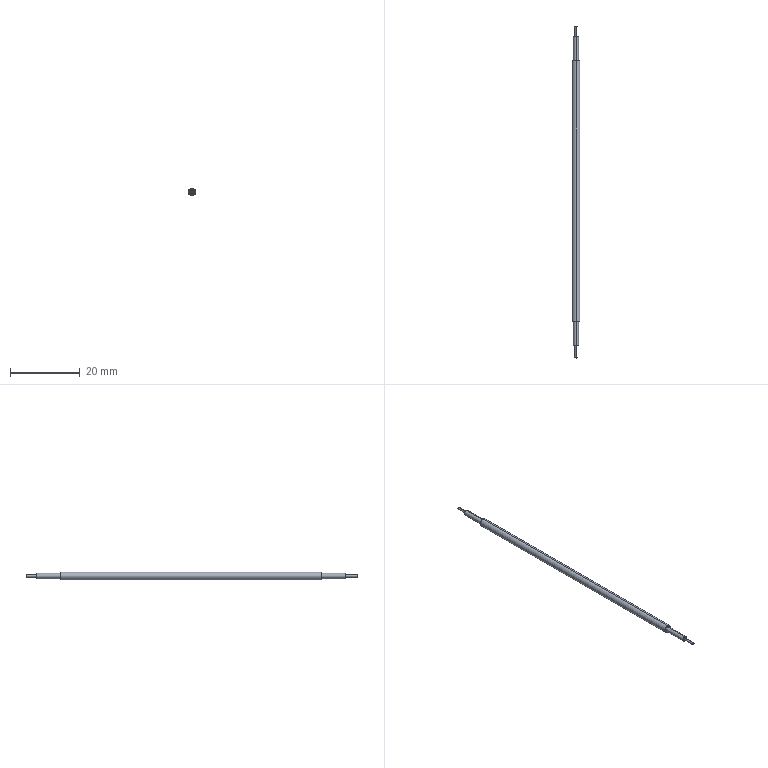Part | SolidWorks | features ICE 4, Extrusion 1 | 1 solid | 16 faces | box 2.25 x 95.2 x 2.25 mm | volume 323.59 mm3 | cylinder 10 | plane 6 | commonest cylinder face diameters 0.6 x4 1.5 x4 2.25 x2
STEP:
#1=CARTESIAN_POINT('',(0.,84.7,0.2999));
#2=VERTEX_POINT('',#1);
#3=CARTESIAN_POINT('',(0.,84.7,-0.2999));
#4=VERTEX_POINT('',#3);
#5=CARTESIAN_POINT('',(0.,84.7,0.));
#6=DIRECTION('',(0.,1.,0.));
#7=DIRECTION('',(0.,0.,1.));
#8=AXIS2_PLACEMENT_3D('',#5,#6,#7);
#9=CIRCLE('',#8,0.2999);
#10=EDGE_CURVE('',#2,#4,#9,.T.);
#11=ORIENTED_EDGE('',*,*,#10,.F.);
#12=CARTESIAN_POINT('',(0.,81.7,0.2999));
#13=VERTEX_POINT('',#12);
#14=CARTESIAN_POINT('',(0.,84.7,0.2999));
#15=DIRECTION('',(0.,-1.,0.));
#16=VECTOR('',#15,1000.);
#17=LINE('',#14,#16);
#18=EDGE_CURVE('',#2,#13,#17,.T.);
#19=ORIENTED_EDGE('',*,*,#18,.T.);
#20=CARTESIAN_POINT('',(0.,81.7,-0.2999));
#21=VERTEX_POINT('',#20);
#22=CARTESIAN_POINT('',(0.,81.7,0.));
#23=DIRECTION('',(0.,1.,0.));
#24=DIRECTION('',(0.,0.,1.));
#25=AXIS2_PLACEMENT_3D('',#22,#23,#24);
#26=CIRCLE('',#25,0.2999);
#27=EDGE_CURVE('',#13,#21,#26,.T.);
#28=ORIENTED_EDGE('',*,*,#27,.T.);
#29=CARTESIAN_POINT('',(0.,84.7,-0.2999));
#30=DIRECTION('',(0.,-1.,0.));
#31=VECTOR('',#30,1000.);
#32=LINE('',#29,#31);
#33=EDGE_CURVE('',#4,#21,#32,.T.);
#34=ORIENTED_EDGE('',*,*,#33,.F.);
#35=EDGE_LOOP('',(#11,#19,#28,#34));
#36=FACE_OUTER_BOUND('',#35,.T.);
#37=CARTESIAN_POINT('',(0.,84.7,0.));
#38=DIRECTION('',(0.,-1.,0.));
#39=DIRECTION('',(0.,0.,-1.));
#40=AXIS2_PLACEMENT_3D('',#37,#38,#39);
#41=CYLINDRICAL_SURFACE('',#40,0.2999);
#42=ADVANCED_FACE('',(#36),#41,.T.);
#43=CARTESIAN_POINT('',(0.,81.7,0.75));
#44=VERTEX_POINT('',#43);
#45=CARTESIAN_POINT('',(0.,81.7,-0.75));
#46=VERTEX_POINT('',#45);
#47=CARTESIAN_POINT('',(0.,81.7,0.));
#48=DIRECTION('',(0.,1.,0.));
#49=DIRECTION('',(0.,0.,1.));
#50=AXIS2_PLACEMENT_3D('',#47,#48,#49);
#51=CIRCLE('',#50,0.75);
#52=EDGE_CURVE('',#44,#46,#51,.T.);
#53=ORIENTED_EDGE('',*,*,#52,.F.);
#54=CARTESIAN_POINT('',(0.,74.7,0.75));
#55=VERTEX_POINT('',#54);
#56=CARTESIAN_POINT('',(0.,81.7,0.75));
#57=DIRECTION('',(0.,-1.,0.));
#58=VECTOR('',#57,1000.);
#59=LINE('',#56,#58);
#60=EDGE_CURVE('',#44,#55,#59,.T.);
#61=ORIENTED_EDGE('',*,*,#60,.T.);
#62=CARTESIAN_POINT('',(0.,74.7,-0.75));
#63=VERTEX_POINT('',#62);
#64=CARTESIAN_POINT('',(0.,74.7,0.));
#65=DIRECTION('',(0.,1.,0.));
#66=DIRECTION('',(0.,0.,1.));
#67=AXIS2_PLACEMENT_3D('',#64,#65,#66);
#68=CIRCLE('',#67,0.75);
#69=EDGE_CURVE('',#55,#63,#68,.T.);
#70=ORIENTED_EDGE('',*,*,#69,.T.);
#71=CARTESIAN_POINT('',(0.,81.7,-0.75));
#72=DIRECTION('',(0.,-1.,0.));
#73=VECTOR('',#72,1000.);
#74=LINE('',#71,#73);
#75=EDGE_CURVE('',#46,#63,#74,.T.);
#76=ORIENTED_EDGE('',*,*,#75,.F.);
#77=EDGE_LOOP('',(#53,#61,#70,#76));
#78=FACE_OUTER_BOUND('',#77,.T.);
#79=CARTESIAN_POINT('',(0.,81.7,0.));
#80=DIRECTION('',(0.,-1.,0.));
#81=DIRECTION('',(0.,0.,-1.));
#82=AXIS2_PLACEMENT_3D('',#79,#80,#81);
#83=CYLINDRICAL_SURFACE('',#82,0.75);
#84=ADVANCED_FACE('',(#78),#83,.T.);
#85=CARTESIAN_POINT('',(0.,-10.5,-0.3));
#86=VERTEX_POINT('',#85);
#87=CARTESIAN_POINT('',(0.,-10.5,0.3));
#88=VERTEX_POINT('',#87);
#89=CARTESIAN_POINT('',(0.,-10.5,0.));
#90=DIRECTION('',(0.,-1.,0.));
#91=DIRECTION('',(0.,0.,-1.));
#92=AXIS2_PLACEMENT_3D('',#89,#90,#91);
#93=CIRCLE('',#92,0.3);
#94=EDGE_CURVE('',#86,#88,#93,.T.);
#95=ORIENTED_EDGE('',*,*,#94,.F.);
#96=CARTESIAN_POINT('',(0.,-7.,-0.3));
#97=VERTEX_POINT('',#96);
#98=CARTESIAN_POINT('',(0.,-10.5,-0.3));
#99=DIRECTION('',(0.,1.,0.));
#100=VECTOR('',#99,1000.);
#101=LINE('',#98,#100);
#102=EDGE_CURVE('',#86,#97,#101,.T.);
#103=ORIENTED_EDGE('',*,*,#102,.T.);
#104=CARTESIAN_POINT('',(0.,-7.,0.3));
#105=VERTEX_POINT('',#104);
#106=CARTESIAN_POINT('',(0.,-7.,0.));
#107=DIRECTION('',(0.,-1.,0.));
#108=DIRECTION('',(0.,0.,-1.));
#109=AXIS2_PLACEMENT_3D('',#106,#107,#108);
#110=CIRCLE('',#109,0.3);
#111=EDGE_CURVE('',#97,#105,#110,.T.);
#112=ORIENTED_EDGE('',*,*,#111,.T.);
#113=CARTESIAN_POINT('',(0.,-10.5,0.3));
#114=DIRECTION('',(0.,1.,0.));
#115=VECTOR('',#114,1000.);
#116=LINE('',#113,#115);
#117=EDGE_CURVE('',#88,#105,#116,.T.);
#118=ORIENTED_EDGE('',*,*,#117,.F.);
#119=EDGE_LOOP('',(#95,#103,#112,#118));
#120=FACE_OUTER_BOUND('',#119,.T.);
#121=CARTESIAN_POINT('',(0.,-10.5,0.));
#122=DIRECTION('',(0.,1.,0.));
#123=DIRECTION('',(0.,0.,1.));
#124=AXIS2_PLACEMENT_3D('',#121,#122,#123);
#125=CYLINDRICAL_SURFACE('',#124,0.3);
#126=ADVANCED_FACE('',(#120),#125,.T.);
#127=CARTESIAN_POINT('',(0.,-7.,-0.75));
#128=VERTEX_POINT('',#127);
#129=CARTESIAN_POINT('',(0.,-7.,0.75));
#130=VERTEX_POINT('',#129);
#131=CARTESIAN_POINT('',(0.,-7.,0.));
#132=DIRECTION('',(0.,-1.,0.));
#133=DIRECTION('',(0.,0.,-1.));
#134=AXIS2_PLACEMENT_3D('',#131,#132,#133);
#135=CIRCLE('',#134,0.75);
#136=EDGE_CURVE('',#128,#130,#135,.T.);
#137=ORIENTED_EDGE('',*,*,#136,.F.);
#138=CARTESIAN_POINT('',(0.,0.,-0.75));
#139=VERTEX_POINT('',#138);
#140=CARTESIAN_POINT('',(0.,-7.,-0.75));
#141=DIRECTION('',(0.,1.,0.));
#142=VECTOR('',#141,1000.);
#143=LINE('',#140,#142);
#144=EDGE_CURVE('',#128,#139,#143,.T.);
#145=ORIENTED_EDGE('',*,*,#144,.T.);
#146=CARTESIAN_POINT('',(0.,0.,0.75));
#147=VERTEX_POINT('',#146);
#148=CARTESIAN_POINT('',(0.,0.,0.));
#149=DIRECTION('',(0.,-1.,0.));
#150=DIRECTION('',(0.,0.,1.));
#151=AXIS2_PLACEMENT_3D('',#148,#149,#150);
#152=CIRCLE('',#151,0.75);
#153=EDGE_CURVE('',#139,#147,#152,.T.);
#154=ORIENTED_EDGE('',*,*,#153,.T.);
#155=CARTESIAN_POINT('',(0.,-7.,0.75));
#156=DIRECTION('',(0.,1.,0.));
#157=VECTOR('',#156,1000.);
#158=LINE('',#155,#157);
#159=EDGE_CURVE('',#130,#147,#158,.T.);
#160=ORIENTED_EDGE('',*,*,#159,.F.);
#161=EDGE_LOOP('',(#137,#145,#154,#160));
#162=FACE_OUTER_BOUND('',#161,.T.);
#163=CARTESIAN_POINT('',(0.,-7.,0.));
#164=DIRECTION('',(0.,1.,0.));
#165=DIRECTION('',(0.,0.,1.));
#166=AXIS2_PLACEMENT_3D('',#163,#164,#165);
#167=CYLINDRICAL_SURFACE('',#166,0.75);
#168=ADVANCED_FACE('',(#162),#167,.T.);
#169=CARTESIAN_POINT('',(0.,74.7,1.125));
#170=VERTEX_POINT('',#169);
#171=CARTESIAN_POINT('',(0.,74.7,-1.125));
#172=VERTEX_POINT('',#171);
#173=CARTESIAN_POINT('',(0.,74.7,0.));
#174=DIRECTION('',(0.,1.,0.));
#175=DIRECTION('',(0.,0.,1.));
#176=AXIS2_PLACEMENT_3D('',#173,#174,#175);
#177=CIRCLE('',#176,1.125);
#178=EDGE_CURVE('',#170,#172,#177,.T.);
#179=ORIENTED_EDGE('',*,*,#178,.F.);
#180=CARTESIAN_POINT('',(0.,0.,1.125));
#181=VERTEX_POINT('',#180);
#182=CARTESIAN_POINT('',(0.,74.7,1.125));
#183=DIRECTION('',(0.,-1.,0.));
#184=VECTOR('',#183,1000.);
#185=LINE('',#182,#184);
#186=EDGE_CURVE('',#170,#181,#185,.T.);
#187=ORIENTED_EDGE('',*,*,#186,.T.);
#188=CARTESIAN_POINT('',(0.,0.,-1.125));
#189=VERTEX_POINT('',#188);
#190=CARTESIAN_POINT('',(0.,0.,0.));
#191=DIRECTION('',(0.,1.,0.));
#192=DIRECTION('',(0.,0.,1.));
#193=AXIS2_PLACEMENT_3D('',#190,#191,#192);
#194=CIRCLE('',#193,1.125);
#195=EDGE_CURVE('',#181,#189,#194,.T.);
#196=ORIENTED_EDGE('',*,*,#195,.T.);
#197=CARTESIAN_POINT('',(0.,74.7,-1.125));
#198=DIRECTION('',(0.,-1.,0.));
#199=VECTOR('',#198,1000.);
#200=LINE('',#197,#199);
#201=EDGE_CURVE('',#172,#189,#200,.T.);
#202=ORIENTED_EDGE('',*,*,#201,.F.);
#203=EDGE_LOOP('',(#179,#187,#196,#202));
#204=FACE_OUTER_BOUND('',#203,.T.);
#205=CARTESIAN_POINT('',(0.,74.7,0.));
#206=DIRECTION('',(0.,-1.,0.));
#207=DIRECTION('',(0.,0.,-1.));
#208=AXIS2_PLACEMENT_3D('',#205,#206,#207);
#209=CYLINDRICAL_SURFACE('',#208,1.125);
#210=ADVANCED_FACE('',(#204),#209,.T.);
#211=CARTESIAN_POINT('',(0.,81.7,0.));
#212=DIRECTION('',(0.,1.,0.));
#213=DIRECTION('',(0.,0.,1.));
#214=AXIS2_PLACEMENT_3D('',#211,#212,#213);
#215=CIRCLE('',#214,0.75);
#216=EDGE_CURVE('',#46,#44,#215,.T.);
#217=ORIENTED_EDGE('',*,*,#216,.T.);
#218=ORIENTED_EDGE('',*,*,#52,.T.);
#219=EDGE_LOOP('',(#217,#218));
#220=FACE_OUTER_BOUND('',#219,.T.);
#221=CARTESIAN_POINT('',(0.,81.7,0.));
#222=DIRECTION('',(0.,1.,0.));
#223=DIRECTION('',(0.,0.,1.));
#224=AXIS2_PLACEMENT_3D('',#221,#222,#223);
#225=CIRCLE('',#224,0.2999);
#226=EDGE_CURVE('',#21,#13,#225,.T.);
#227=ORIENTED_EDGE('',*,*,#226,.F.);
#228=ORIENTED_EDGE('',*,*,#27,.F.);
#229=EDGE_LOOP('',(#227,#228));
#230=FACE_BOUND('',#229,.T.);
#231=CARTESIAN_POINT('',(0.,81.7,0.));
#232=DIRECTION('',(0.,1.,0.));
#233=DIRECTION('',(0.,0.,1.));
#234=AXIS2_PLACEMENT_3D('',#231,#232,#233);
#235=PLANE('',#234);
#236=ADVANCED_FACE('',(#220,#230),#235,.T.);
#237=CARTESIAN_POINT('',(0.,74.7,0.));
#238=DIRECTION('',(0.,1.,0.));
#239=DIRECTION('',(0.,0.,1.));
#240=AXIS2_PLACEMENT_3D('',#237,#238,#239);
#241=CIRCLE('',#240,1.125);
#242=EDGE_CURVE('',#172,#170,#241,.T.);
#243=ORIENTED_EDGE('',*,*,#242,.T.);
#244=ORIENTED_EDGE('',*,*,#178,.T.);
#245=EDGE_LOOP('',(#243,#244));
#246=FACE_OUTER_BOUND('',#245,.T.);
#247=CARTESIAN_POINT('',(0.,74.7,0.));
#248=DIRECTION('',(0.,1.,0.));
#249=DIRECTION('',(0.,0.,1.));
#250=AXIS2_PLACEMENT_3D('',#247,#248,#249);
#251=CIRCLE('',#250,0.75);
#252=EDGE_CURVE('',#63,#55,#251,.T.);
#253=ORIENTED_EDGE('',*,*,#252,.F.);
#254=ORIENTED_EDGE('',*,*,#69,.F.);
#255=EDGE_LOOP('',(#253,#254));
#256=FACE_BOUND('',#255,.T.);
#257=CARTESIAN_POINT('',(0.,74.7,0.));
#258=DIRECTION('',(0.,1.,0.));
#259=DIRECTION('',(0.,0.,1.));
#260=AXIS2_PLACEMENT_3D('',#257,#258,#259);
#261=PLANE('',#260);
#262=ADVANCED_FACE('',(#246,#256),#261,.T.);
#263=CARTESIAN_POINT('',(0.,-7.,0.));
#264=DIRECTION('',(0.,-1.,0.));
#265=DIRECTION('',(0.,0.,-1.));
#266=AXIS2_PLACEMENT_3D('',#263,#264,#265);
#267=CIRCLE('',#266,0.75);
#268=EDGE_CURVE('',#130,#128,#267,.T.);
#269=ORIENTED_EDGE('',*,*,#268,.T.);
#270=ORIENTED_EDGE('',*,*,#136,.T.);
#271=EDGE_LOOP('',(#269,#270));
#272=FACE_OUTER_BOUND('',#271,.T.);
#273=CARTESIAN_POINT('',(0.,-7.,0.));
#274=DIRECTION('',(0.,-1.,0.));
#275=DIRECTION('',(0.,0.,-1.));
#276=AXIS2_PLACEMENT_3D('',#273,#274,#275);
#277=CIRCLE('',#276,0.3);
#278=EDGE_CURVE('',#105,#97,#277,.T.);
#279=ORIENTED_EDGE('',*,*,#278,.F.);
#280=ORIENTED_EDGE('',*,*,#111,.F.);
#281=EDGE_LOOP('',(#279,#280));
#282=FACE_BOUND('',#281,.T.);
#283=CARTESIAN_POINT('',(0.,-7.,0.));
#284=DIRECTION('',(0.,-1.,0.));
#285=DIRECTION('',(0.,0.,-1.));
#286=AXIS2_PLACEMENT_3D('',#283,#284,#285);
#287=PLANE('',#286);
#288=ADVANCED_FACE('',(#272,#282),#287,.T.);
#289=CARTESIAN_POINT('',(0.,0.,0.));
#290=DIRECTION('',(0.,1.,0.));
#291=DIRECTION('',(0.,0.,1.));
#292=AXIS2_PLACEMENT_3D('',#289,#290,#291);
#293=CIRCLE('',#292,1.125);
#294=EDGE_CURVE('',#189,#181,#293,.T.);
#295=ORIENTED_EDGE('',*,*,#294,.F.);
#296=ORIENTED_EDGE('',*,*,#195,.F.);
#297=EDGE_LOOP('',(#295,#296));
#298=FACE_OUTER_BOUND('',#297,.T.);
#299=CARTESIAN_POINT('',(0.,0.,0.));
#300=DIRECTION('',(0.,-1.,0.));
#301=DIRECTION('',(0.,0.,1.));
#302=AXIS2_PLACEMENT_3D('',#299,#300,#301);
#303=CIRCLE('',#302,0.75);
#304=EDGE_CURVE('',#147,#139,#303,.T.);
#305=ORIENTED_EDGE('',*,*,#304,.F.);
#306=ORIENTED_EDGE('',*,*,#153,.F.);
#307=EDGE_LOOP('',(#305,#306));
#308=FACE_BOUND('',#307,.T.);
#309=CARTESIAN_POINT('',(0.,0.,0.));
#310=DIRECTION('',(0.,1.,0.));
#311=DIRECTION('',(0.,0.,1.));
#312=AXIS2_PLACEMENT_3D('',#309,#310,#311);
#313=PLANE('',#312);
#314=ADVANCED_FACE('',(#298,#308),#313,.F.);
#315=ORIENTED_EDGE('',*,*,#186,.F.);
#316=ORIENTED_EDGE('',*,*,#242,.F.);
#317=ORIENTED_EDGE('',*,*,#201,.T.);
#318=ORIENTED_EDGE('',*,*,#294,.T.);
#319=EDGE_LOOP('',(#315,#316,#317,#318));
#320=FACE_OUTER_BOUND('',#319,.T.);
#321=CARTESIAN_POINT('',(0.,74.7,0.));
#322=DIRECTION('',(0.,-1.,0.));
#323=DIRECTION('',(0.,0.,-1.));
#324=AXIS2_PLACEMENT_3D('',#321,#322,#323);
#325=CYLINDRICAL_SURFACE('',#324,1.125);
#326=ADVANCED_FACE('',(#320),#325,.T.);
#327=ORIENTED_EDGE('',*,*,#144,.F.);
#328=ORIENTED_EDGE('',*,*,#268,.F.);
#329=ORIENTED_EDGE('',*,*,#159,.T.);
#330=ORIENTED_EDGE('',*,*,#304,.T.);
#331=EDGE_LOOP('',(#327,#328,#329,#330));
#332=FACE_OUTER_BOUND('',#331,.T.);
#333=CARTESIAN_POINT('',(0.,-7.,0.));
#334=DIRECTION('',(0.,1.,0.));
#335=DIRECTION('',(0.,0.,1.));
#336=AXIS2_PLACEMENT_3D('',#333,#334,#335);
#337=CYLINDRICAL_SURFACE('',#336,0.75);
#338=ADVANCED_FACE('',(#332),#337,.T.);
#339=ORIENTED_EDGE('',*,*,#102,.F.);
#340=CARTESIAN_POINT('',(0.,-10.5,0.));
#341=DIRECTION('',(0.,-1.,0.));
#342=DIRECTION('',(0.,0.,-1.));
#343=AXIS2_PLACEMENT_3D('',#340,#341,#342);
#344=CIRCLE('',#343,0.3);
#345=EDGE_CURVE('',#88,#86,#344,.T.);
#346=ORIENTED_EDGE('',*,*,#345,.F.);
#347=ORIENTED_EDGE('',*,*,#117,.T.);
#348=ORIENTED_EDGE('',*,*,#278,.T.);
#349=EDGE_LOOP('',(#339,#346,#347,#348));
#350=FACE_OUTER_BOUND('',#349,.T.);
#351=CARTESIAN_POINT('',(0.,-10.5,0.));
#352=DIRECTION('',(0.,1.,0.));
#353=DIRECTION('',(0.,0.,1.));
#354=AXIS2_PLACEMENT_3D('',#351,#352,#353);
#355=CYLINDRICAL_SURFACE('',#354,0.3);
#356=ADVANCED_FACE('',(#350),#355,.T.);
#357=ORIENTED_EDGE('',*,*,#345,.T.);
#358=ORIENTED_EDGE('',*,*,#94,.T.);
#359=EDGE_LOOP('',(#357,#358));
#360=FACE_OUTER_BOUND('',#359,.T.);
#361=CARTESIAN_POINT('',(0.,-10.5,0.));
#362=DIRECTION('',(0.,-1.,0.));
#363=DIRECTION('',(0.,0.,-1.));
#364=AXIS2_PLACEMENT_3D('',#361,#362,#363);
#365=PLANE('',#364);
#366=ADVANCED_FACE('',(#360),#365,.T.);
#367=ORIENTED_EDGE('',*,*,#60,.F.);
#368=ORIENTED_EDGE('',*,*,#216,.F.);
#369=ORIENTED_EDGE('',*,*,#75,.T.);
#370=ORIENTED_EDGE('',*,*,#252,.T.);
#371=EDGE_LOOP('',(#367,#368,#369,#370));
#372=FACE_OUTER_BOUND('',#371,.T.);
#373=CARTESIAN_POINT('',(0.,81.7,0.));
#374=DIRECTION('',(0.,-1.,0.));
#375=DIRECTION('',(0.,0.,-1.));
#376=AXIS2_PLACEMENT_3D('',#373,#374,#375);
#377=CYLINDRICAL_SURFACE('',#376,0.75);
#378=ADVANCED_FACE('',(#372),#377,.T.);
#379=ORIENTED_EDGE('',*,*,#18,.F.);
#380=CARTESIAN_POINT('',(0.,84.7,0.));
#381=DIRECTION('',(0.,1.,0.));
#382=DIRECTION('',(0.,0.,1.));
#383=AXIS2_PLACEMENT_3D('',#380,#381,#382);
#384=CIRCLE('',#383,0.2999);
#385=EDGE_CURVE('',#4,#2,#384,.T.);
#386=ORIENTED_EDGE('',*,*,#385,.F.);
#387=ORIENTED_EDGE('',*,*,#33,.T.);
#388=ORIENTED_EDGE('',*,*,#226,.T.);
#389=EDGE_LOOP('',(#379,#386,#387,#388));
#390=FACE_OUTER_BOUND('',#389,.T.);
#391=CARTESIAN_POINT('',(0.,84.7,0.));
#392=DIRECTION('',(0.,-1.,0.));
#393=DIRECTION('',(0.,0.,-1.));
#394=AXIS2_PLACEMENT_3D('',#391,#392,#393);
#395=CYLINDRICAL_SURFACE('',#394,0.2999);
#396=ADVANCED_FACE('',(#390),#395,.T.);
#397=ORIENTED_EDGE('',*,*,#385,.T.);
#398=ORIENTED_EDGE('',*,*,#10,.T.);
#399=EDGE_LOOP('',(#397,#398));
#400=FACE_OUTER_BOUND('',#399,.T.);
#401=CARTESIAN_POINT('',(0.,84.7,0.));
#402=DIRECTION('',(0.,1.,0.));
#403=DIRECTION('',(0.,0.,1.));
#404=AXIS2_PLACEMENT_3D('',#401,#402,#403);
#405=PLANE('',#404);
#406=ADVANCED_FACE('',(#400),#405,.T.);
#407=CLOSED_SHELL('',(#42,#84,#126,#168,#210,#236,#262,#288,#314,#326,#338,#356,#366,#378,#396,#406));
#408=MANIFOLD_SOLID_BREP('',#407);
#409=CARTESIAN_POINT('',(0.,0.,0.));
#410=DIRECTION('',(0.,0.,1.));
#411=DIRECTION('',(1.,0.,0.));
#412=AXIS2_PLACEMENT_3D('',#409,#410,#411);
#413=(LENGTH_UNIT()NAMED_UNIT(*)SI_UNIT(.MILLI.,.METRE.));
#414=UNCERTAINTY_MEASURE_WITH_UNIT(LENGTH_MEASURE(0.00001),#413,'','');
#415=(NAMED_UNIT(*)PLANE_ANGLE_UNIT()SI_UNIT($,.RADIAN.));
#416=(NAMED_UNIT(*)SI_UNIT($,.STERADIAN.)SOLID_ANGLE_UNIT());
#417=(GEOMETRIC_REPRESENTATION_CONTEXT(3)GLOBAL_UNCERTAINTY_ASSIGNED_CONTEXT((#414))GLOBAL_UNIT_ASSIGNED_CONTEXT((#413,#415,#416))REPRESENTATION_CONTEXT('',''));
#418=ADVANCED_BREP_SHAPE_REPRESENTATION('',(#408,#412),#417);